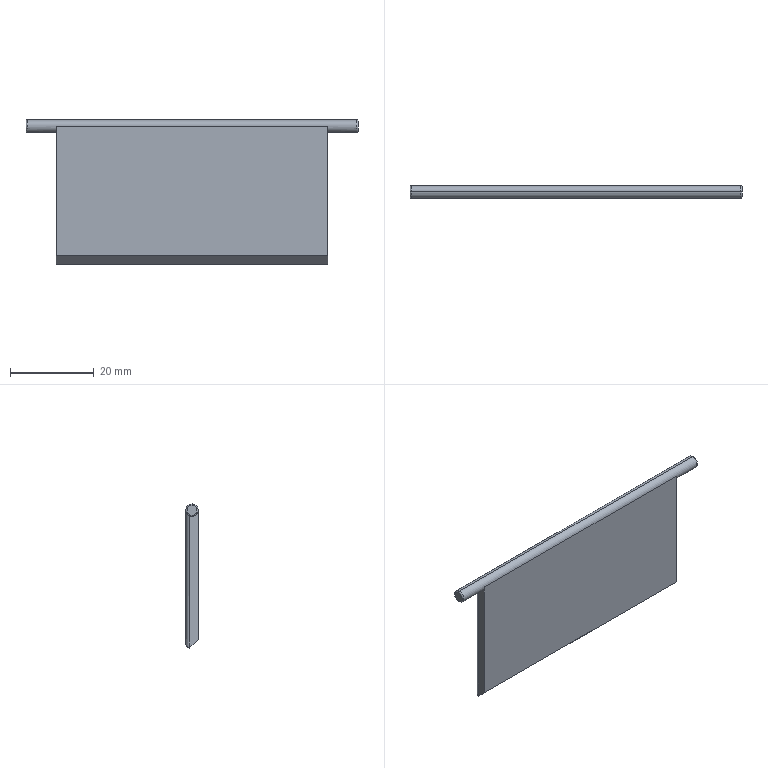Part | SolidWorks | features Fillet 2, Chamfer 1, Extrusion 1, ICE 1 | 1 solid | 16 faces | box 79.5 x 3 x 34.5 mm | volume 6609 mm3 | plane 7 | cylinder 5 | torus 4 | commonest cylinder face diameters 2 x3 3 x2
STEP:
#1=CARTESIAN_POINT('',(-39.75,1.5,17.7));
#2=VERTEX_POINT('',#1);
#3=CARTESIAN_POINT('',(-39.75,1.5,15.3));
#4=VERTEX_POINT('',#3);
#5=CARTESIAN_POINT('',(-39.75,1.5,16.5));
#6=DIRECTION('',(-1.,0.,0.));
#7=DIRECTION('',(0.,0.,-1.));
#8=AXIS2_PLACEMENT_3D('',#5,#6,#7);
#9=CIRCLE('',#8,1.2);
#10=EDGE_CURVE('',#2,#4,#9,.T.);
#11=ORIENTED_EDGE('',*,*,#10,.F.);
#12=CARTESIAN_POINT('',(-39.45,1.5,18.));
#13=VERTEX_POINT('',#12);
#14=CARTESIAN_POINT('',(-39.45,1.5,17.7));
#15=DIRECTION('',(0.,1.,0.));
#16=DIRECTION('',(0.,0.,1.));
#17=AXIS2_PLACEMENT_3D('',#14,#15,#16);
#18=CIRCLE('',#17,0.3);
#19=EDGE_CURVE('',#2,#13,#18,.T.);
#20=ORIENTED_EDGE('',*,*,#19,.T.);
#21=CARTESIAN_POINT('',(-39.45,1.5,15.));
#22=VERTEX_POINT('',#21);
#23=CARTESIAN_POINT('',(-39.45,1.5,16.5));
#24=DIRECTION('',(1.,0.,0.));
#25=DIRECTION('',(0.,0.,-1.));
#26=AXIS2_PLACEMENT_3D('',#23,#24,#25);
#27=CIRCLE('',#26,1.5);
#28=EDGE_CURVE('',#22,#13,#27,.T.);
#29=ORIENTED_EDGE('',*,*,#28,.F.);
#30=CARTESIAN_POINT('',(-39.45,1.5,15.3));
#31=DIRECTION('',(0.,-1.,0.));
#32=DIRECTION('',(0.,0.,-1.));
#33=AXIS2_PLACEMENT_3D('',#30,#31,#32);
#34=CIRCLE('',#33,0.3);
#35=EDGE_CURVE('',#4,#22,#34,.T.);
#36=ORIENTED_EDGE('',*,*,#35,.F.);
#37=EDGE_LOOP('',(#11,#20,#29,#36));
#38=FACE_OUTER_BOUND('',#37,.T.);
#39=CARTESIAN_POINT('',(-39.45,1.5,16.5));
#40=DIRECTION('',(1.,0.,0.));
#41=DIRECTION('',(0.,0.,-1.));
#42=AXIS2_PLACEMENT_3D('',#39,#40,#41);
#43=TOROIDAL_SURFACE('',#42,1.2,0.3);
#44=ADVANCED_FACE('',(#38),#43,.T.);
#45=CARTESIAN_POINT('',(39.45,1.5,18.));
#46=VERTEX_POINT('',#45);
#47=CARTESIAN_POINT('',(39.45,1.5,15.));
#48=VERTEX_POINT('',#47);
#49=CARTESIAN_POINT('',(39.45,1.5,16.5));
#50=DIRECTION('',(-1.,0.,0.));
#51=DIRECTION('',(0.,0.,-1.));
#52=AXIS2_PLACEMENT_3D('',#49,#50,#51);
#53=CIRCLE('',#52,1.5);
#54=EDGE_CURVE('',#46,#48,#53,.T.);
#55=ORIENTED_EDGE('',*,*,#54,.F.);
#56=CARTESIAN_POINT('',(39.75,1.5,17.7));
#57=VERTEX_POINT('',#56);
#58=CARTESIAN_POINT('',(39.45,1.5,17.7));
#59=DIRECTION('',(0.,1.,0.));
#60=DIRECTION('',(0.,0.,1.));
#61=AXIS2_PLACEMENT_3D('',#58,#59,#60);
#62=CIRCLE('',#61,0.3);
#63=EDGE_CURVE('',#46,#57,#62,.T.);
#64=ORIENTED_EDGE('',*,*,#63,.T.);
#65=CARTESIAN_POINT('',(39.75,1.5,15.3));
#66=VERTEX_POINT('',#65);
#67=CARTESIAN_POINT('',(39.75,1.5,16.5));
#68=DIRECTION('',(1.,0.,0.));
#69=DIRECTION('',(0.,0.,-1.));
#70=AXIS2_PLACEMENT_3D('',#67,#68,#69);
#71=CIRCLE('',#70,1.2);
#72=EDGE_CURVE('',#66,#57,#71,.T.);
#73=ORIENTED_EDGE('',*,*,#72,.F.);
#74=CARTESIAN_POINT('',(39.45,1.5,15.3));
#75=DIRECTION('',(0.,-1.,0.));
#76=DIRECTION('',(0.,0.,-1.));
#77=AXIS2_PLACEMENT_3D('',#74,#75,#76);
#78=CIRCLE('',#77,0.3);
#79=EDGE_CURVE('',#48,#66,#78,.T.);
#80=ORIENTED_EDGE('',*,*,#79,.F.);
#81=EDGE_LOOP('',(#55,#64,#73,#80));
#82=FACE_OUTER_BOUND('',#81,.T.);
#83=CARTESIAN_POINT('',(39.45,1.5,16.5));
#84=DIRECTION('',(1.,0.,0.));
#85=DIRECTION('',(0.,0.,-1.));
#86=AXIS2_PLACEMENT_3D('',#83,#84,#85);
#87=TOROIDAL_SURFACE('',#86,1.2,0.3);
#88=ADVANCED_FACE('',(#82),#87,.T.);
#89=ORIENTED_EDGE('',*,*,#54,.T.);
#90=CARTESIAN_POINT('',(32.5,1.5,15.));
#91=VERTEX_POINT('',#90);
#92=CARTESIAN_POINT('',(39.75,1.5,15.));
#93=DIRECTION('',(-1.,0.,0.));
#94=VECTOR('',#93,1000.);
#95=LINE('',#92,#94);
#96=EDGE_CURVE('',#48,#91,#95,.T.);
#97=ORIENTED_EDGE('',*,*,#96,.T.);
#98=CARTESIAN_POINT('',(32.5,2.,15.086));
#99=VERTEX_POINT('',#98);
#100=CARTESIAN_POINT('',(32.5,1.5,16.5));
#101=DIRECTION('',(1.,0.,0.));
#102=DIRECTION('',(0.,0.,1.));
#103=AXIS2_PLACEMENT_3D('',#100,#101,#102);
#104=CIRCLE('',#103,1.5);
#105=EDGE_CURVE('',#91,#99,#104,.T.);
#106=ORIENTED_EDGE('',*,*,#105,.T.);
#107=CARTESIAN_POINT('',(31.5,3.,16.5));
#108=VERTEX_POINT('',#107);
#109=CARTESIAN_POINT('',(32.5,2.,15.086));
#110=CARTESIAN_POINT('',(32.5,2.085,15.116));
#111=CARTESIAN_POINT('',(32.489,2.166,15.153));
#112=CARTESIAN_POINT('',(32.452,2.317,15.239));
#113=CARTESIAN_POINT('',(32.424,2.389,15.289));
#114=CARTESIAN_POINT('',(32.327,2.58,15.446));
#115=CARTESIAN_POINT('',(32.239,2.685,15.568));
#116=CARTESIAN_POINT('',(32.049,2.845,15.82));
#117=CARTESIAN_POINT('',(31.942,2.904,15.954));
#118=CARTESIAN_POINT('',(31.725,2.981,16.224));
#119=CARTESIAN_POINT('',(31.612,3.,16.362));
#120=CARTESIAN_POINT('',(31.5,3.,16.5));
#121=B_SPLINE_CURVE_WITH_KNOTS('',3,(#109,#110,#111,#112,#113,#114,#115,#116,#117,#118,#119,#120),.UNSPECIFIED.,.F.,.F.,(4,2,2,2,2,4),(0.,0.0002668,0.0005336,0.001067,0.001601,0.002134),.UNSPECIFIED.);
#122=EDGE_CURVE('',#99,#108,#121,.T.);
#123=ORIENTED_EDGE('',*,*,#122,.T.);
#124=CARTESIAN_POINT('',(-31.5,3.,16.5));
#125=VERTEX_POINT('',#124);
#126=CARTESIAN_POINT('',(-32.5,3.,16.5));
#127=DIRECTION('',(1.,0.,0.));
#128=VECTOR('',#127,1000.);
#129=LINE('',#126,#128);
#130=EDGE_CURVE('',#125,#108,#129,.T.);
#131=ORIENTED_EDGE('',*,*,#130,.F.);
#132=CARTESIAN_POINT('',(-32.5,2.,15.086));
#133=VERTEX_POINT('',#132);
#134=CARTESIAN_POINT('',(-31.5,3.,16.5));
#135=CARTESIAN_POINT('',(-31.612,3.,16.363));
#136=CARTESIAN_POINT('',(-31.725,2.981,16.224));
#137=CARTESIAN_POINT('',(-31.942,2.904,15.954));
#138=CARTESIAN_POINT('',(-32.049,2.845,15.82));
#139=CARTESIAN_POINT('',(-32.239,2.685,15.568));
#140=CARTESIAN_POINT('',(-32.327,2.58,15.446));
#141=CARTESIAN_POINT('',(-32.424,2.389,15.289));
#142=CARTESIAN_POINT('',(-32.452,2.317,15.239));
#143=CARTESIAN_POINT('',(-32.489,2.166,15.153));
#144=CARTESIAN_POINT('',(-32.5,2.085,15.116));
#145=CARTESIAN_POINT('',(-32.5,2.,15.086));
#146=B_SPLINE_CURVE_WITH_KNOTS('',3,(#134,#135,#136,#137,#138,#139,#140,#141,#142,#143,#144,#145),.UNSPECIFIED.,.F.,.F.,(4,2,2,2,2,4),(-0.000007746,0.000524,0.001056,0.001588,0.001853,0.002119),.UNSPECIFIED.);
#147=EDGE_CURVE('',#125,#133,#146,.T.);
#148=ORIENTED_EDGE('',*,*,#147,.T.);
#149=CARTESIAN_POINT('',(-32.5,1.5,15.));
#150=VERTEX_POINT('',#149);
#151=CARTESIAN_POINT('',(-32.5,1.5,16.5));
#152=DIRECTION('',(-1.,0.,0.));
#153=DIRECTION('',(0.,0.,-1.));
#154=AXIS2_PLACEMENT_3D('',#151,#152,#153);
#155=CIRCLE('',#154,1.5);
#156=EDGE_CURVE('',#133,#150,#155,.T.);
#157=ORIENTED_EDGE('',*,*,#156,.T.);
#158=CARTESIAN_POINT('',(39.75,1.5,15.));
#159=DIRECTION('',(-1.,0.,0.));
#160=VECTOR('',#159,1000.);
#161=LINE('',#158,#160);
#162=EDGE_CURVE('',#150,#22,#161,.T.);
#163=ORIENTED_EDGE('',*,*,#162,.T.);
#164=ORIENTED_EDGE('',*,*,#28,.T.);
#165=CARTESIAN_POINT('',(39.75,1.5,18.));
#166=DIRECTION('',(-1.,0.,0.));
#167=VECTOR('',#166,1000.);
#168=LINE('',#165,#167);
#169=EDGE_CURVE('',#46,#13,#168,.T.);
#170=ORIENTED_EDGE('',*,*,#169,.F.);
#171=EDGE_LOOP('',(#89,#97,#106,#123,#131,#148,#157,#163,#164,#170));
#172=FACE_OUTER_BOUND('',#171,.T.);
#173=CARTESIAN_POINT('',(39.75,1.5,16.5));
#174=DIRECTION('',(-1.,0.,0.));
#175=DIRECTION('',(0.,0.,1.));
#176=AXIS2_PLACEMENT_3D('',#173,#174,#175);
#177=CYLINDRICAL_SURFACE('',#176,1.5);
#178=ADVANCED_FACE('',(#172),#177,.T.);
#179=CARTESIAN_POINT('',(32.5,0.,-14.5));
#180=VERTEX_POINT('',#179);
#181=CARTESIAN_POINT('',(32.5,2.,-16.5));
#182=VERTEX_POINT('',#181);
#183=CARTESIAN_POINT('',(32.5,2.,-16.5));
#184=DIRECTION('',(0.,0.7071,-0.7071));
#185=VECTOR('',#184,1000.);
#186=LINE('',#183,#185);
#187=EDGE_CURVE('',#180,#182,#186,.T.);
#188=ORIENTED_EDGE('',*,*,#187,.T.);
#189=CARTESIAN_POINT('',(32.5,2.,16.5));
#190=DIRECTION('',(0.,0.,1.));
#191=VECTOR('',#190,1000.);
#192=LINE('',#189,#191);
#193=EDGE_CURVE('',#182,#99,#192,.T.);
#194=ORIENTED_EDGE('',*,*,#193,.T.);
#195=ORIENTED_EDGE('',*,*,#105,.F.);
#196=CARTESIAN_POINT('',(32.5,0.,16.5));
#197=VERTEX_POINT('',#196);
#198=CARTESIAN_POINT('',(32.5,1.5,16.5));
#199=DIRECTION('',(1.,0.,0.));
#200=DIRECTION('',(0.,0.,1.));
#201=AXIS2_PLACEMENT_3D('',#198,#199,#200);
#202=CIRCLE('',#201,1.5);
#203=EDGE_CURVE('',#197,#91,#202,.T.);
#204=ORIENTED_EDGE('',*,*,#203,.F.);
#205=CARTESIAN_POINT('',(32.5,0.,-16.5));
#206=DIRECTION('',(0.,0.,-1.));
#207=VECTOR('',#206,1000.);
#208=LINE('',#205,#207);
#209=EDGE_CURVE('',#197,#180,#208,.T.);
#210=ORIENTED_EDGE('',*,*,#209,.T.);
#211=EDGE_LOOP('',(#188,#194,#195,#204,#210));
#212=FACE_OUTER_BOUND('',#211,.T.);
#213=CARTESIAN_POINT('',(32.5,3.,-16.5));
#214=DIRECTION('',(-1.,0.,0.));
#215=DIRECTION('',(0.,0.,1.));
#216=AXIS2_PLACEMENT_3D('',#213,#214,#215);
#217=PLANE('',#216);
#218=ADVANCED_FACE('',(#212),#217,.F.);
#219=ORIENTED_EDGE('',*,*,#156,.F.);
#220=CARTESIAN_POINT('',(-32.5,2.,-16.5));
#221=VERTEX_POINT('',#220);
#222=CARTESIAN_POINT('',(-32.5,2.,-16.5));
#223=DIRECTION('',(0.,0.,-1.));
#224=VECTOR('',#223,1000.);
#225=LINE('',#222,#224);
#226=EDGE_CURVE('',#133,#221,#225,.T.);
#227=ORIENTED_EDGE('',*,*,#226,.T.);
#228=CARTESIAN_POINT('',(-32.5,0.,-14.5));
#229=VERTEX_POINT('',#228);
#230=CARTESIAN_POINT('',(-32.5,2.,-16.5));
#231=DIRECTION('',(0.,-0.7071,0.7071));
#232=VECTOR('',#231,1000.);
#233=LINE('',#230,#232);
#234=EDGE_CURVE('',#221,#229,#233,.T.);
#235=ORIENTED_EDGE('',*,*,#234,.T.);
#236=CARTESIAN_POINT('',(-32.5,0.,16.5));
#237=VERTEX_POINT('',#236);
#238=CARTESIAN_POINT('',(-32.5,0.,-16.5));
#239=DIRECTION('',(0.,0.,1.));
#240=VECTOR('',#239,1000.);
#241=LINE('',#238,#240);
#242=EDGE_CURVE('',#229,#237,#241,.T.);
#243=ORIENTED_EDGE('',*,*,#242,.T.);
#244=CARTESIAN_POINT('',(-32.5,1.5,16.5));
#245=DIRECTION('',(-1.,0.,0.));
#246=DIRECTION('',(0.,0.,-1.));
#247=AXIS2_PLACEMENT_3D('',#244,#245,#246);
#248=CIRCLE('',#247,1.5);
#249=EDGE_CURVE('',#150,#237,#248,.T.);
#250=ORIENTED_EDGE('',*,*,#249,.F.);
#251=EDGE_LOOP('',(#219,#227,#235,#243,#250));
#252=FACE_OUTER_BOUND('',#251,.T.);
#253=CARTESIAN_POINT('',(-32.5,3.,-16.5));
#254=DIRECTION('',(1.,0.,0.));
#255=DIRECTION('',(0.,0.,-1.));
#256=AXIS2_PLACEMENT_3D('',#253,#254,#255);
#257=PLANE('',#256);
#258=ADVANCED_FACE('',(#252),#257,.F.);
#259=ORIENTED_EDGE('',*,*,#130,.T.);
#260=CARTESIAN_POINT('',(31.5,3.,-15.5));
#261=VERTEX_POINT('',#260);
#262=CARTESIAN_POINT('',(31.5,3.,-16.5));
#263=DIRECTION('',(0.,0.,-1.));
#264=VECTOR('',#263,1000.);
#265=LINE('',#262,#264);
#266=EDGE_CURVE('',#108,#261,#265,.T.);
#267=ORIENTED_EDGE('',*,*,#266,.T.);
#268=CARTESIAN_POINT('',(-31.5,3.,-15.5));
#269=VERTEX_POINT('',#268);
#270=CARTESIAN_POINT('',(-32.5,3.,-15.5));
#271=DIRECTION('',(-1.,0.,0.));
#272=VECTOR('',#271,1000.);
#273=LINE('',#270,#272);
#274=EDGE_CURVE('',#261,#269,#273,.T.);
#275=ORIENTED_EDGE('',*,*,#274,.T.);
#276=CARTESIAN_POINT('',(-31.5,3.,16.5));
#277=DIRECTION('',(0.,0.,1.));
#278=VECTOR('',#277,1000.);
#279=LINE('',#276,#278);
#280=EDGE_CURVE('',#269,#125,#279,.T.);
#281=ORIENTED_EDGE('',*,*,#280,.T.);
#282=EDGE_LOOP('',(#259,#267,#275,#281));
#283=FACE_OUTER_BOUND('',#282,.T.);
#284=CARTESIAN_POINT('',(0.,3.,0.));
#285=DIRECTION('',(0.,1.,0.));
#286=DIRECTION('',(0.,0.,1.));
#287=AXIS2_PLACEMENT_3D('',#284,#285,#286);
#288=PLANE('',#287);
#289=ADVANCED_FACE('',(#283),#288,.T.);
#290=ORIENTED_EDGE('',*,*,#242,.F.);
#291=CARTESIAN_POINT('',(0.,0.,-14.5));
#292=DIRECTION('',(1.,0.,0.));
#293=VECTOR('',#292,1000.);
#294=LINE('',#291,#293);
#295=EDGE_CURVE('',#229,#180,#294,.T.);
#296=ORIENTED_EDGE('',*,*,#295,.T.);
#297=ORIENTED_EDGE('',*,*,#209,.F.);
#298=CARTESIAN_POINT('',(-32.5,0.,16.5));
#299=DIRECTION('',(1.,0.,0.));
#300=VECTOR('',#299,1000.);
#301=LINE('',#298,#300);
#302=EDGE_CURVE('',#237,#197,#301,.T.);
#303=ORIENTED_EDGE('',*,*,#302,.F.);
#304=EDGE_LOOP('',(#290,#296,#297,#303));
#305=FACE_OUTER_BOUND('',#304,.T.);
#306=CARTESIAN_POINT('',(0.,0.,0.));
#307=DIRECTION('',(0.,1.,0.));
#308=DIRECTION('',(0.,0.,1.));
#309=AXIS2_PLACEMENT_3D('',#306,#307,#308);
#310=PLANE('',#309);
#311=ADVANCED_FACE('',(#305),#310,.F.);
#312=ORIENTED_EDGE('',*,*,#96,.F.);
#313=CARTESIAN_POINT('',(39.45,1.5,16.5));
#314=DIRECTION('',(-1.,0.,0.));
#315=DIRECTION('',(0.,0.,-1.));
#316=AXIS2_PLACEMENT_3D('',#313,#314,#315);
#317=CIRCLE('',#316,1.5);
#318=EDGE_CURVE('',#48,#46,#317,.T.);
#319=ORIENTED_EDGE('',*,*,#318,.T.);
#320=ORIENTED_EDGE('',*,*,#169,.T.);
#321=CARTESIAN_POINT('',(-39.45,1.5,16.5));
#322=DIRECTION('',(1.,0.,0.));
#323=DIRECTION('',(0.,0.,-1.));
#324=AXIS2_PLACEMENT_3D('',#321,#322,#323);
#325=CIRCLE('',#324,1.5);
#326=EDGE_CURVE('',#13,#22,#325,.T.);
#327=ORIENTED_EDGE('',*,*,#326,.T.);
#328=ORIENTED_EDGE('',*,*,#162,.F.);
#329=ORIENTED_EDGE('',*,*,#249,.T.);
#330=ORIENTED_EDGE('',*,*,#302,.T.);
#331=ORIENTED_EDGE('',*,*,#203,.T.);
#332=EDGE_LOOP('',(#312,#319,#320,#327,#328,#329,#330,#331));
#333=FACE_OUTER_BOUND('',#332,.T.);
#334=CARTESIAN_POINT('',(39.75,1.5,16.5));
#335=DIRECTION('',(-1.,0.,0.));
#336=DIRECTION('',(0.,0.,1.));
#337=AXIS2_PLACEMENT_3D('',#334,#335,#336);
#338=CYLINDRICAL_SURFACE('',#337,1.5);
#339=ADVANCED_FACE('',(#333),#338,.T.);
#340=ORIENTED_EDGE('',*,*,#72,.T.);
#341=CARTESIAN_POINT('',(39.75,1.5,16.5));
#342=DIRECTION('',(1.,0.,0.));
#343=DIRECTION('',(0.,0.,-1.));
#344=AXIS2_PLACEMENT_3D('',#341,#342,#343);
#345=CIRCLE('',#344,1.2);
#346=EDGE_CURVE('',#57,#66,#345,.T.);
#347=ORIENTED_EDGE('',*,*,#346,.T.);
#348=EDGE_LOOP('',(#340,#347));
#349=FACE_OUTER_BOUND('',#348,.T.);
#350=CARTESIAN_POINT('',(39.75,1.5,16.5));
#351=DIRECTION('',(1.,0.,0.));
#352=DIRECTION('',(0.,0.,-1.));
#353=AXIS2_PLACEMENT_3D('',#350,#351,#352);
#354=PLANE('',#353);
#355=ADVANCED_FACE('',(#349),#354,.T.);
#356=CARTESIAN_POINT('',(-39.75,1.5,16.5));
#357=DIRECTION('',(-1.,0.,0.));
#358=DIRECTION('',(0.,0.,-1.));
#359=AXIS2_PLACEMENT_3D('',#356,#357,#358);
#360=CIRCLE('',#359,1.2);
#361=EDGE_CURVE('',#4,#2,#360,.T.);
#362=ORIENTED_EDGE('',*,*,#361,.T.);
#363=ORIENTED_EDGE('',*,*,#10,.T.);
#364=EDGE_LOOP('',(#362,#363));
#365=FACE_OUTER_BOUND('',#364,.T.);
#366=CARTESIAN_POINT('',(-39.75,1.5,16.5));
#367=DIRECTION('',(1.,0.,0.));
#368=DIRECTION('',(0.,0.,-1.));
#369=AXIS2_PLACEMENT_3D('',#366,#367,#368);
#370=PLANE('',#369);
#371=ADVANCED_FACE('',(#365),#370,.F.);
#372=ORIENTED_EDGE('',*,*,#187,.F.);
#373=ORIENTED_EDGE('',*,*,#295,.F.);
#374=ORIENTED_EDGE('',*,*,#234,.F.);
#375=CARTESIAN_POINT('',(-32.5,2.,-16.5));
#376=DIRECTION('',(-1.,0.,0.));
#377=VECTOR('',#376,1000.);
#378=LINE('',#375,#377);
#379=EDGE_CURVE('',#182,#221,#378,.T.);
#380=ORIENTED_EDGE('',*,*,#379,.F.);
#381=EDGE_LOOP('',(#372,#373,#374,#380));
#382=FACE_OUTER_BOUND('',#381,.T.);
#383=CARTESIAN_POINT('',(-32.5,2.,-16.5));
#384=DIRECTION('',(0.,0.7071,0.7071));
#385=DIRECTION('',(-1.,0.,0.));
#386=AXIS2_PLACEMENT_3D('',#383,#384,#385);
#387=PLANE('',#386);
#388=ADVANCED_FACE('',(#382),#387,.F.);
#389=ORIENTED_EDGE('',*,*,#147,.F.);
#390=ORIENTED_EDGE('',*,*,#280,.F.);
#391=CARTESIAN_POINT('',(-32.5,2.,-16.5));
#392=CARTESIAN_POINT('',(-32.5,2.586,-16.5));
#393=CARTESIAN_POINT('',(-32.086,3.,-16.086));
#394=CARTESIAN_POINT('',(-31.5,3.,-15.5));
#395=(BOUNDED_CURVE()B_SPLINE_CURVE(3,(#391,#392,#393,#394),.UNSPECIFIED.,.F.,.F.)B_SPLINE_CURVE_WITH_KNOTS((4,4),(3.142,4.712),.UNSPECIFIED.)CURVE()GEOMETRIC_REPRESENTATION_ITEM()RATIONAL_B_SPLINE_CURVE((1.,0.8047,0.8047,1.))REPRESENTATION_ITEM(''));
#396=EDGE_CURVE('',#221,#269,#395,.T.);
#397=ORIENTED_EDGE('',*,*,#396,.F.);
#398=ORIENTED_EDGE('',*,*,#226,.F.);
#399=EDGE_LOOP('',(#389,#390,#397,#398));
#400=FACE_OUTER_BOUND('',#399,.T.);
#401=CARTESIAN_POINT('',(-31.5,2.,0.));
#402=DIRECTION('',(0.,0.,-1.));
#403=DIRECTION('',(-1.,0.,0.));
#404=AXIS2_PLACEMENT_3D('',#401,#402,#403);
#405=CYLINDRICAL_SURFACE('',#404,1.);
#406=ADVANCED_FACE('',(#400),#405,.T.);
#407=ORIENTED_EDGE('',*,*,#396,.T.);
#408=ORIENTED_EDGE('',*,*,#274,.F.);
#409=CARTESIAN_POINT('',(32.5,2.,-16.5));
#410=CARTESIAN_POINT('',(32.5,2.586,-16.5));
#411=CARTESIAN_POINT('',(32.086,3.,-16.086));
#412=CARTESIAN_POINT('',(31.5,3.,-15.5));
#413=(BOUNDED_CURVE()B_SPLINE_CURVE(3,(#409,#410,#411,#412),.UNSPECIFIED.,.F.,.F.)B_SPLINE_CURVE_WITH_KNOTS((4,4),(0.,1.571),.UNSPECIFIED.)CURVE()GEOMETRIC_REPRESENTATION_ITEM()RATIONAL_B_SPLINE_CURVE((1.,0.8047,0.8047,1.))REPRESENTATION_ITEM(''));
#414=EDGE_CURVE('',#182,#261,#413,.T.);
#415=ORIENTED_EDGE('',*,*,#414,.F.);
#416=ORIENTED_EDGE('',*,*,#379,.T.);
#417=EDGE_LOOP('',(#407,#408,#415,#416));
#418=FACE_OUTER_BOUND('',#417,.T.);
#419=CARTESIAN_POINT('',(0.,2.,-15.5));
#420=DIRECTION('',(1.,0.,0.));
#421=DIRECTION('',(0.,0.,-1.));
#422=AXIS2_PLACEMENT_3D('',#419,#420,#421);
#423=CYLINDRICAL_SURFACE('',#422,1.);
#424=ADVANCED_FACE('',(#418),#423,.T.);
#425=ORIENTED_EDGE('',*,*,#122,.F.);
#426=ORIENTED_EDGE('',*,*,#193,.F.);
#427=ORIENTED_EDGE('',*,*,#414,.T.);
#428=ORIENTED_EDGE('',*,*,#266,.F.);
#429=EDGE_LOOP('',(#425,#426,#427,#428));
#430=FACE_OUTER_BOUND('',#429,.T.);
#431=CARTESIAN_POINT('',(31.5,2.,0.));
#432=DIRECTION('',(0.,0.,1.));
#433=DIRECTION('',(1.,0.,0.));
#434=AXIS2_PLACEMENT_3D('',#431,#432,#433);
#435=CYLINDRICAL_SURFACE('',#434,1.);
#436=ADVANCED_FACE('',(#430),#435,.T.);
#437=ORIENTED_EDGE('',*,*,#63,.F.);
#438=ORIENTED_EDGE('',*,*,#318,.F.);
#439=ORIENTED_EDGE('',*,*,#79,.T.);
#440=ORIENTED_EDGE('',*,*,#346,.F.);
#441=EDGE_LOOP('',(#437,#438,#439,#440));
#442=FACE_OUTER_BOUND('',#441,.T.);
#443=CARTESIAN_POINT('',(39.45,1.5,16.5));
#444=DIRECTION('',(1.,0.,0.));
#445=DIRECTION('',(0.,0.,-1.));
#446=AXIS2_PLACEMENT_3D('',#443,#444,#445);
#447=TOROIDAL_SURFACE('',#446,1.2,0.3);
#448=ADVANCED_FACE('',(#442),#447,.T.);
#449=ORIENTED_EDGE('',*,*,#19,.F.);
#450=ORIENTED_EDGE('',*,*,#361,.F.);
#451=ORIENTED_EDGE('',*,*,#35,.T.);
#452=ORIENTED_EDGE('',*,*,#326,.F.);
#453=EDGE_LOOP('',(#449,#450,#451,#452));
#454=FACE_OUTER_BOUND('',#453,.T.);
#455=CARTESIAN_POINT('',(-39.45,1.5,16.5));
#456=DIRECTION('',(1.,0.,0.));
#457=DIRECTION('',(0.,0.,-1.));
#458=AXIS2_PLACEMENT_3D('',#455,#456,#457);
#459=TOROIDAL_SURFACE('',#458,1.2,0.3);
#460=ADVANCED_FACE('',(#454),#459,.T.);
#461=CLOSED_SHELL('',(#44,#88,#178,#218,#258,#289,#311,#339,#355,#371,#388,#406,#424,#436,#448,#460));
#462=MANIFOLD_SOLID_BREP('',#461);
#463=CARTESIAN_POINT('',(0.,0.,0.));
#464=DIRECTION('',(0.,0.,1.));
#465=DIRECTION('',(1.,0.,0.));
#466=AXIS2_PLACEMENT_3D('',#463,#464,#465);
#467=(LENGTH_UNIT()NAMED_UNIT(*)SI_UNIT(.MILLI.,.METRE.));
#468=UNCERTAINTY_MEASURE_WITH_UNIT(LENGTH_MEASURE(0.00001),#467,'','');
#469=(NAMED_UNIT(*)PLANE_ANGLE_UNIT()SI_UNIT($,.RADIAN.));
#470=(NAMED_UNIT(*)SI_UNIT($,.STERADIAN.)SOLID_ANGLE_UNIT());
#471=(GEOMETRIC_REPRESENTATION_CONTEXT(3)GLOBAL_UNCERTAINTY_ASSIGNED_CONTEXT((#468))GLOBAL_UNIT_ASSIGNED_CONTEXT((#467,#469,#470))REPRESENTATION_CONTEXT('',''));
#472=ADVANCED_BREP_SHAPE_REPRESENTATION('',(#462,#466),#471);